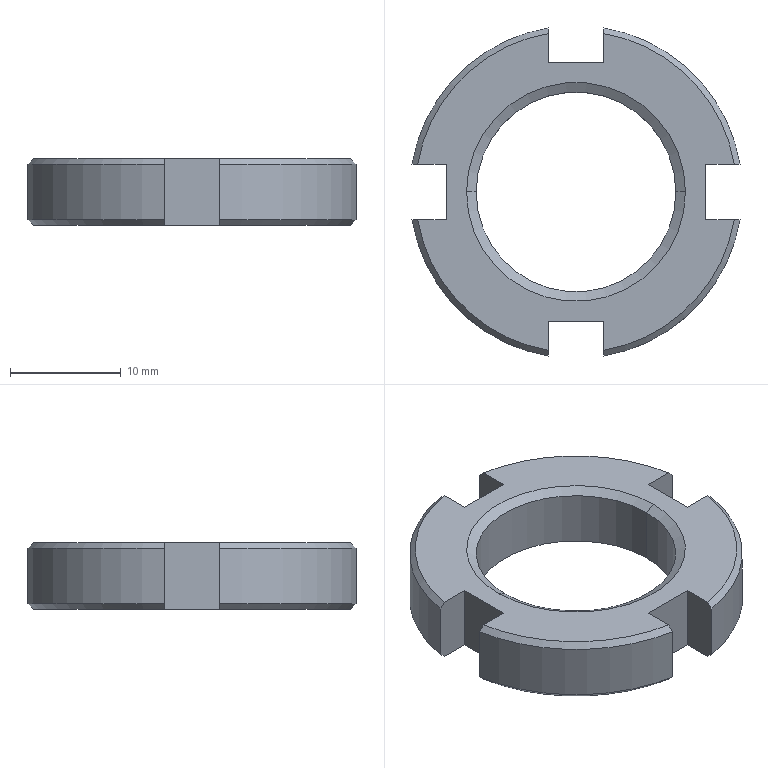Part | STEP file | GB/T810-1988 small round nut M18x1.5 | 1 solid | 32 faces | box 29.58 x 29.58 x 6 mm | volume 2282 mm3 | plane 14 | cone 12 | cylinder 6 | commonest cylinder face diameters 30 x4 18 x2